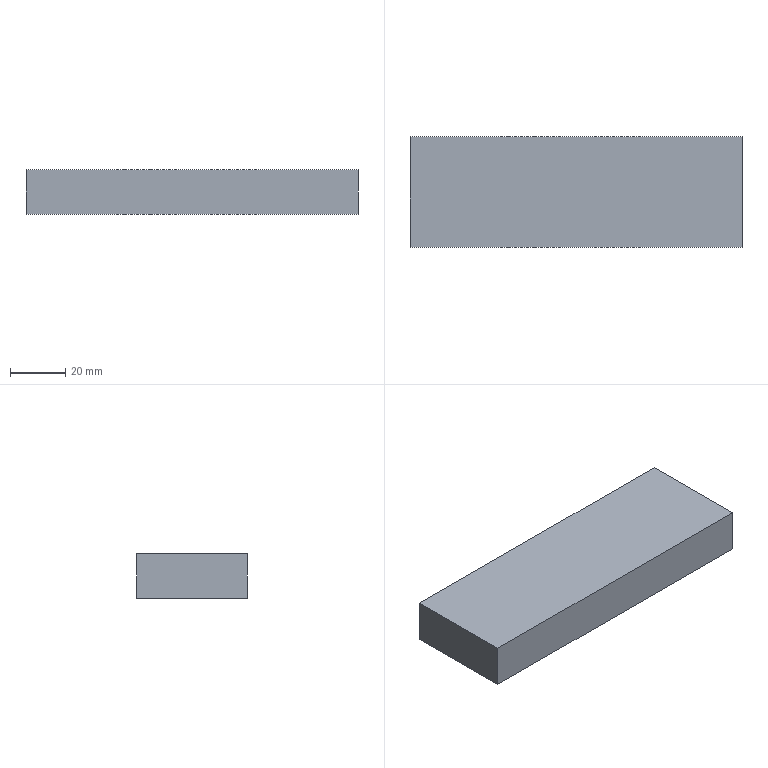Part | SolidWorks | features Extrusion 1 | 1 solid | 6 faces | box 120 x 40 x 16 mm | volume 76800 mm3 | plane 6
STEP:
#1=CARTESIAN_POINT('',(60.,-20.,-8.));
#2=VERTEX_POINT('',#1);
#3=CARTESIAN_POINT('',(60.,20.,-8.));
#4=VERTEX_POINT('',#3);
#5=CARTESIAN_POINT('',(60.,-20.,-8.));
#6=DIRECTION('',(0.,1.,0.));
#7=VECTOR('',#6,1000.);
#8=LINE('',#5,#7);
#9=EDGE_CURVE('',#2,#4,#8,.T.);
#10=ORIENTED_EDGE('',*,*,#9,.T.);
#11=CARTESIAN_POINT('',(60.,20.,8.));
#12=VERTEX_POINT('',#11);
#13=CARTESIAN_POINT('',(60.,20.,8.));
#14=DIRECTION('',(0.,0.,-1.));
#15=VECTOR('',#14,1000.);
#16=LINE('',#13,#15);
#17=EDGE_CURVE('',#12,#4,#16,.T.);
#18=ORIENTED_EDGE('',*,*,#17,.F.);
#19=CARTESIAN_POINT('',(60.,-20.,8.));
#20=VERTEX_POINT('',#19);
#21=CARTESIAN_POINT('',(60.,-20.,8.));
#22=DIRECTION('',(0.,1.,0.));
#23=VECTOR('',#22,1000.);
#24=LINE('',#21,#23);
#25=EDGE_CURVE('',#20,#12,#24,.T.);
#26=ORIENTED_EDGE('',*,*,#25,.F.);
#27=CARTESIAN_POINT('',(60.,-20.,8.));
#28=DIRECTION('',(0.,0.,-1.));
#29=VECTOR('',#28,1000.);
#30=LINE('',#27,#29);
#31=EDGE_CURVE('',#20,#2,#30,.T.);
#32=ORIENTED_EDGE('',*,*,#31,.T.);
#33=EDGE_LOOP('',(#10,#18,#26,#32));
#34=FACE_OUTER_BOUND('',#33,.T.);
#35=CARTESIAN_POINT('',(60.,-20.,8.));
#36=DIRECTION('',(-1.,0.,0.));
#37=DIRECTION('',(0.,0.,1.));
#38=AXIS2_PLACEMENT_3D('',#35,#36,#37);
#39=PLANE('',#38);
#40=ADVANCED_FACE('',(#34),#39,.F.);
#41=CARTESIAN_POINT('',(-60.,20.,-8.));
#42=VERTEX_POINT('',#41);
#43=CARTESIAN_POINT('',(-60.,20.,-8.));
#44=DIRECTION('',(-1.,0.,0.));
#45=VECTOR('',#44,1000.);
#46=LINE('',#43,#45);
#47=EDGE_CURVE('',#4,#42,#46,.T.);
#48=ORIENTED_EDGE('',*,*,#47,.T.);
#49=CARTESIAN_POINT('',(-60.,20.,8.));
#50=VERTEX_POINT('',#49);
#51=CARTESIAN_POINT('',(-60.,20.,8.));
#52=DIRECTION('',(0.,0.,-1.));
#53=VECTOR('',#52,1000.);
#54=LINE('',#51,#53);
#55=EDGE_CURVE('',#50,#42,#54,.T.);
#56=ORIENTED_EDGE('',*,*,#55,.F.);
#57=CARTESIAN_POINT('',(-60.,20.,8.));
#58=DIRECTION('',(-1.,0.,0.));
#59=VECTOR('',#58,1000.);
#60=LINE('',#57,#59);
#61=EDGE_CURVE('',#12,#50,#60,.T.);
#62=ORIENTED_EDGE('',*,*,#61,.F.);
#63=ORIENTED_EDGE('',*,*,#17,.T.);
#64=EDGE_LOOP('',(#48,#56,#62,#63));
#65=FACE_OUTER_BOUND('',#64,.T.);
#66=CARTESIAN_POINT('',(-60.,20.,8.));
#67=DIRECTION('',(0.,-1.,0.));
#68=DIRECTION('',(0.,0.,-1.));
#69=AXIS2_PLACEMENT_3D('',#66,#67,#68);
#70=PLANE('',#69);
#71=ADVANCED_FACE('',(#65),#70,.F.);
#72=CARTESIAN_POINT('',(-60.,-20.,-8.));
#73=VERTEX_POINT('',#72);
#74=CARTESIAN_POINT('',(-60.,-20.,-8.));
#75=DIRECTION('',(0.,-1.,0.));
#76=VECTOR('',#75,1000.);
#77=LINE('',#74,#76);
#78=EDGE_CURVE('',#42,#73,#77,.T.);
#79=ORIENTED_EDGE('',*,*,#78,.T.);
#80=CARTESIAN_POINT('',(-60.,-20.,8.));
#81=VERTEX_POINT('',#80);
#82=CARTESIAN_POINT('',(-60.,-20.,8.));
#83=DIRECTION('',(0.,0.,-1.));
#84=VECTOR('',#83,1000.);
#85=LINE('',#82,#84);
#86=EDGE_CURVE('',#81,#73,#85,.T.);
#87=ORIENTED_EDGE('',*,*,#86,.F.);
#88=CARTESIAN_POINT('',(-60.,-20.,8.));
#89=DIRECTION('',(0.,-1.,0.));
#90=VECTOR('',#89,1000.);
#91=LINE('',#88,#90);
#92=EDGE_CURVE('',#50,#81,#91,.T.);
#93=ORIENTED_EDGE('',*,*,#92,.F.);
#94=ORIENTED_EDGE('',*,*,#55,.T.);
#95=EDGE_LOOP('',(#79,#87,#93,#94));
#96=FACE_OUTER_BOUND('',#95,.T.);
#97=CARTESIAN_POINT('',(-60.,-20.,8.));
#98=DIRECTION('',(1.,0.,0.));
#99=DIRECTION('',(0.,0.,-1.));
#100=AXIS2_PLACEMENT_3D('',#97,#98,#99);
#101=PLANE('',#100);
#102=ADVANCED_FACE('',(#96),#101,.F.);
#103=CARTESIAN_POINT('',(-60.,-20.,-8.));
#104=DIRECTION('',(1.,0.,0.));
#105=VECTOR('',#104,1000.);
#106=LINE('',#103,#105);
#107=EDGE_CURVE('',#73,#2,#106,.T.);
#108=ORIENTED_EDGE('',*,*,#107,.T.);
#109=ORIENTED_EDGE('',*,*,#31,.F.);
#110=CARTESIAN_POINT('',(-60.,-20.,8.));
#111=DIRECTION('',(1.,0.,0.));
#112=VECTOR('',#111,1000.);
#113=LINE('',#110,#112);
#114=EDGE_CURVE('',#81,#20,#113,.T.);
#115=ORIENTED_EDGE('',*,*,#114,.F.);
#116=ORIENTED_EDGE('',*,*,#86,.T.);
#117=EDGE_LOOP('',(#108,#109,#115,#116));
#118=FACE_OUTER_BOUND('',#117,.T.);
#119=CARTESIAN_POINT('',(-60.,-20.,8.));
#120=DIRECTION('',(0.,1.,0.));
#121=DIRECTION('',(0.,0.,1.));
#122=AXIS2_PLACEMENT_3D('',#119,#120,#121);
#123=PLANE('',#122);
#124=ADVANCED_FACE('',(#118),#123,.F.);
#125=ORIENTED_EDGE('',*,*,#25,.T.);
#126=ORIENTED_EDGE('',*,*,#61,.T.);
#127=ORIENTED_EDGE('',*,*,#92,.T.);
#128=ORIENTED_EDGE('',*,*,#114,.T.);
#129=EDGE_LOOP('',(#125,#126,#127,#128));
#130=FACE_OUTER_BOUND('',#129,.T.);
#131=CARTESIAN_POINT('',(0.,0.,8.));
#132=DIRECTION('',(0.,0.,-1.));
#133=DIRECTION('',(-1.,0.,0.));
#134=AXIS2_PLACEMENT_3D('',#131,#132,#133);
#135=PLANE('',#134);
#136=ADVANCED_FACE('',(#130),#135,.F.);
#137=ORIENTED_EDGE('',*,*,#9,.F.);
#138=ORIENTED_EDGE('',*,*,#107,.F.);
#139=ORIENTED_EDGE('',*,*,#78,.F.);
#140=ORIENTED_EDGE('',*,*,#47,.F.);
#141=EDGE_LOOP('',(#137,#138,#139,#140));
#142=FACE_OUTER_BOUND('',#141,.T.);
#143=CARTESIAN_POINT('',(0.,0.,-8.));
#144=DIRECTION('',(0.,0.,-1.));
#145=DIRECTION('',(-1.,0.,0.));
#146=AXIS2_PLACEMENT_3D('',#143,#144,#145);
#147=PLANE('',#146);
#148=ADVANCED_FACE('',(#142),#147,.T.);
#149=CLOSED_SHELL('',(#40,#71,#102,#124,#136,#148));
#150=MANIFOLD_SOLID_BREP('',#149);
#151=CARTESIAN_POINT('',(0.,0.,0.));
#152=DIRECTION('',(0.,0.,1.));
#153=DIRECTION('',(1.,0.,0.));
#154=AXIS2_PLACEMENT_3D('',#151,#152,#153);
#155=(LENGTH_UNIT()NAMED_UNIT(*)SI_UNIT(.MILLI.,.METRE.));
#156=UNCERTAINTY_MEASURE_WITH_UNIT(LENGTH_MEASURE(0.00001),#155,'','');
#157=(NAMED_UNIT(*)PLANE_ANGLE_UNIT()SI_UNIT($,.RADIAN.));
#158=(NAMED_UNIT(*)SI_UNIT($,.STERADIAN.)SOLID_ANGLE_UNIT());
#159=(GEOMETRIC_REPRESENTATION_CONTEXT(3)GLOBAL_UNCERTAINTY_ASSIGNED_CONTEXT((#156))GLOBAL_UNIT_ASSIGNED_CONTEXT((#155,#157,#158))REPRESENTATION_CONTEXT('',''));
#160=ADVANCED_BREP_SHAPE_REPRESENTATION('',(#150,#154),#159);